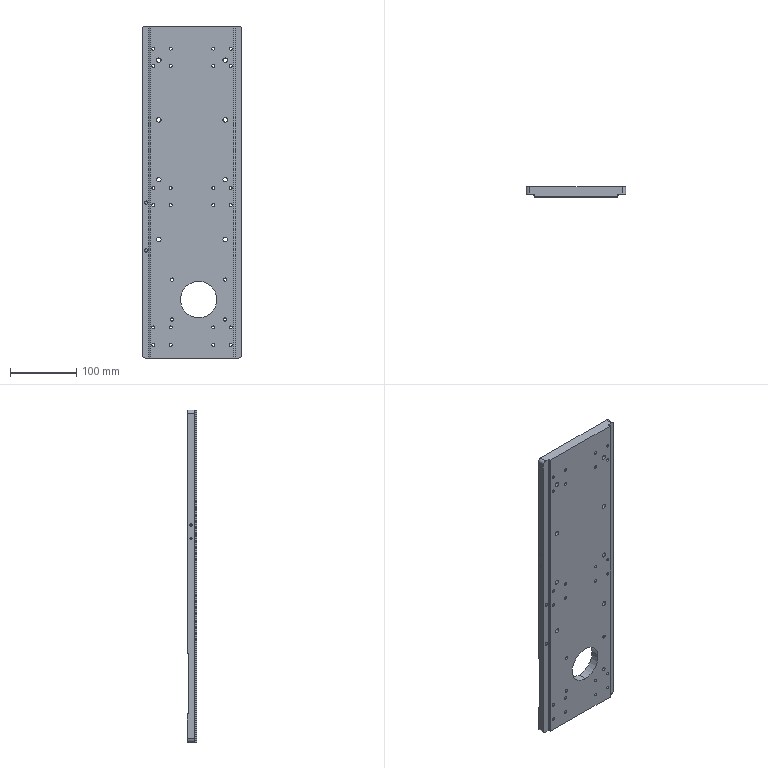Part | SolidWorks | features BaseBody 1 | 1 solid | 200 faces | box 150 x 15 x 500 mm | volume 1000700 mm3 | cylinder 144 | plane 44 | cone 12 | commonest cylinder face diameters 4.5 x48 8 x48 6.8 x16 5 x12 3.3 x8 6 x4